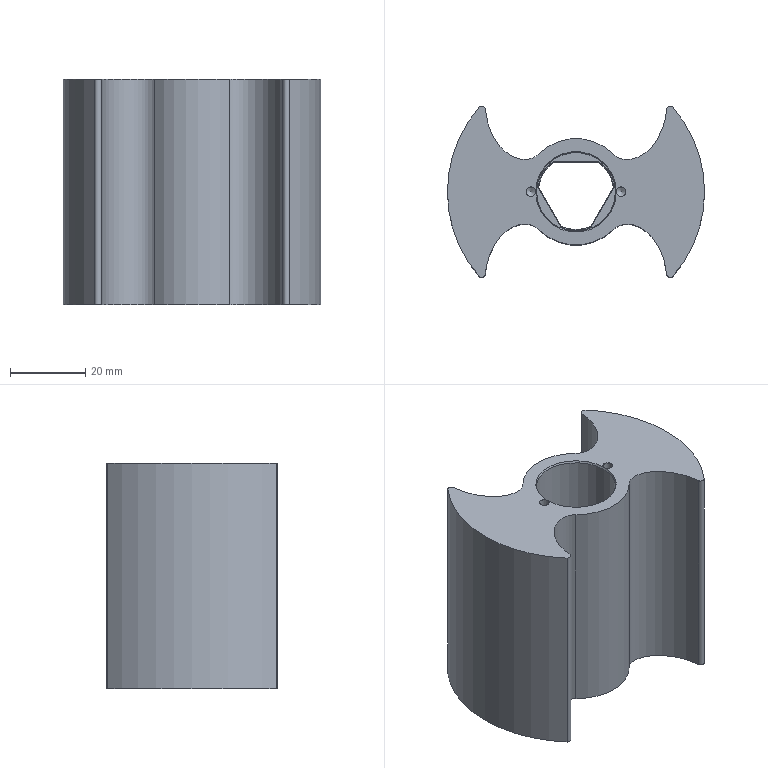CAM job | NX | 3-axis milling, drilling | part box 68.489 x 45.577 x 60 mm | stock box 68.489 x 68.489 x 60 mm
Tools:
number,name,description,diameter,corner_radius,flute_length,length,flutes
1,ZXZ,Milling Tool-5 Parameters,6.0,0.0,50.0,75.0,2
12,2.5ZT,Drilling Tool,2.5,0.0,35.0,50.0,2
12,D12,Milling Tool-5 Parameters,12.0,0.0,50.0,75.0,2
5,D25R0.5,Milling Tool-5 Parameters,25.0,0.5,50.0,75.0,2
7,D6A45,Milling Tool-5 Parameters,6.0,0.0,50.0,75.0,2
Operations:
program,operation,operation_type,tool,method,geometry_group,spindle_rpm,surface_speed,feed_per_tooth,feed_cut,feed_plunge,cut_length_mm,path_length_mm,cut_time_min,machine_time_min
1,DRILLING_COPY_1,Operation,ZXZ,METHOD,A,5000.0,94.0,0.025,250.0,0.0,8.0,103.187,0.032,0.0415
1,DRILLING_COPY_1_COPY,Operation,2.5ZT,METHOD,A,2000.0,15.0,0.03,120.0,0.0,15.502,118.191,0.1292,0.1395
1,ZLEVEL_PROFILE_COPY_1,ZLevelMilling,D12,METHOD,A,3000.0,113.0,0.3,1800.0,1000.0,3524.546,3644.246,2.012,2.024
1,CUTTERCOMP12_1,ZLevelMilling,D12,METHOD,A,5000.0,157.0,0.125,1250.0,100.0,985.792,5475.507,0.7886,1.238
2,ZLEVEL_PROFILE_COPY_2,ZLevelMilling,D25R0.5,METHOD,A,2000.0,157.0,0.55,2200.0,1000.0,36793.573,110937.473,17.995,25.41
2,CUTTERCOMP12,ZLevelMilling,D12,METHOD,A,5000.0,157.0,0.125,1250.0,100.0,11105.186,33007.358,8.884,11.074
2,PLANAR_MILL_COPY_COPY,PlanarMilling,D6A45,METHOD,A,7500.0,141.0,0.0833,1250.0,100.0,255.317,312.317,0.2043,0.21